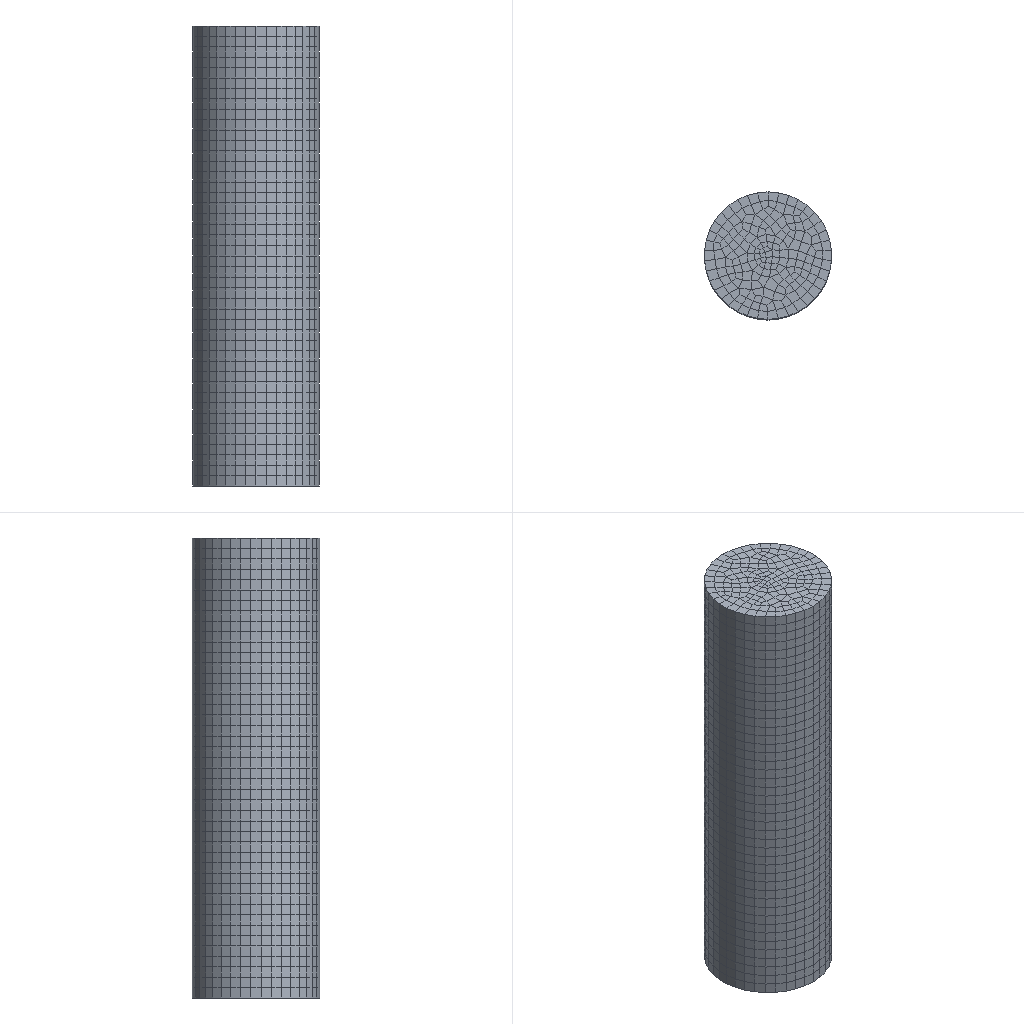Simulation study | abaqus
Set-up summary:
category,name,step,type,value,unit,region
solver,abaqus
solver,version,,,Abaqus/Standard 2020
units,not stated in the deck,,not stated
analysis,deck,,coupled temperature-displacement,coupled temperature-displacement
load_step,Step-1,Step-1,coupled temperature-displacement
load_step,requested,,,1
mesh,nodes,,,9270
mesh,elements,,,8184
element_type,C3D8RT,,solid,8184
load,load commands in deck,,count,2
bc,support commands in deck,,count,1
material,MATERIAL-1,,in results
check,setup vs results,,match,"per instance, exact: element labels, types and connectivity; labels of the nodes the elements use; coordinates of those nodes at SINGLE_PRECISION in 1 of 1 instance(s)"
Abaqus input file, long lists of numbers shortened:
*Heading
** Job name: Job-1 Model name: Model-1
** Generated by: Abaqus/CAE 2020
*Preprint, echo=NO, model=NO, history=NO, contact=NO
**
** PARTS
**
*Part, name=Part-1
*Node
      1,   5.525,  -7.104,          25.
      2,   1.543,  -2.572,          25.
** (9268 more lines like these left out)
*Element, type=C3D8RT
   1, 2958, 2987,  691,  692,  210,  239,   10,   11
   2, 2988, 3021, 3029, 2958,  240,  273,  281,  210
** (8182 more lines like these left out)
*Nset, nset=Set-1, generate
    1,  9270,     1
*Elset, elset=Set-1, generate
    1,  8184,     1
** Section: Section-1
*Solid Section, elset=Set-1, material=Material-1
,
*End Part
**
**
** ASSEMBLY
**
*Assembly, name=Assembly
**
*Instance, name=Part-1-1, part=Part-1
*End Instance
**
*Nset, nset=Set-1, instance=Part-1-1
    2,    5,   46,   47,   48,   49,   50,   51,   52,   53,   54,   55,   56,   57,   58,  109
  110,  111,  112,  113,  114,  115,  116,  117,  118,  119,  120,  121, 1767, 1768, 1769, 1770
** (26 more lines like these left out)
*Elset, elset=Set-1, instance=Part-1-1, generate
 7321,  7640,     1
*Nset, nset=Set-2, instance=Part-1-1
    3,    4,   59,   60,   61,   62,   63,   64,   65,   66,   67,   68,   69,   70,   71,   72
   73,   74,   75,   76,   77,   78,   79,   80,   81,   82,   83,   84,   85,   86,   87,   88
** (11 more lines like these left out)
*Elset, elset=Set-2, instance=Part-1-1
 2465, 2466, 2467, 2468, 2469, 2470, 2471, 2472, 2473, 2474, 2475, 2476, 2477, 2478, 2479, 2480
 2481, 2482, 2483, 2484, 2485, 2486, 2487, 2488, 2489, 2490, 2491, 2492, 2493, 2494, 2495, 2496
** (10 more lines like these left out)
*Elset, elset=_Surf-1_S1, internal, instance=Part-1-1, generate
 7289,  7320,     1
*Surface, type=ELEMENT, name=Surf-1
_Surf-1_S1, S1
*End Assembly
*Amplitude, name=Amp-1, definition=PERIODIC
1,            6.28,              0.,              1.
             1.,              0.
*Amplitude, name=Amp-2
             0.,              0.,             10.,              1.
**
** MATERIALS
**
*Material, name=Material-1
*Conductivity
45.,
*Density
 7.8e-09,
*Elastic
210000., 0.3
*Expansion
 1.5e-05,
*Specific Heat
 4.6e+08,
** ----------------------------------------------------------------
**
** STEP: Step-1
**
*Step, name=Step-1, nlgeom=YES, inc=10000
*Coupled Temperature-displacement, creep=none, deltmx=1e+06, stabilize=0.0002, allsdtol=0.05, continue=NO
1., 1000., 0.01, 1000.
**
** BOUNDARY CONDITIONS
**
** Name: BC-1 Type: 位移/转角
*Boundary
Set-2, 3, 3
**
** LOADS
**
** Name: Load-1   Type: Body heat flux
*Dflux, amplitude=Amp-2
Set-1, BF, 40.
** Name: Load-2   Type: Pressure
*Dsload, amplitude=Amp-1
Surf-1, P, 100.
**
** OUTPUT REQUESTS
**
*Restart, write, frequency=0
**
** FIELD OUTPUT: F-Output-1
**
*Output, field
*Node Output
CF, NT, RF, RFL, RM, RT, TF, U
UR, UT, V, VR, VT
*Element Output, directions=YES
E, HFL, LE, MISES, MISESMAX, MISESONLY, PE, PEEQ, PEEQMAX, PEEQT, PEMAG, S, SF, SSAVG, TEMP, YIELDPOT
*Contact Output
CDISP, CSTRESS
*Radiation Output
FTEMP,
**
** HISTORY OUTPUT: H-Output-1
**
*Output, history, variable=PRESELECT
*End Step
Results summary:
result,step,,completed,increments=17 time=1000.0/1000.0
result,analysis,,,"coupled temperature-displacement, steady state"
result,last_loadstep,,,1
result,primary field,,,"U, NT11"
result,reaction total,,FX,0.0,model units
result,reaction total,,FY,0.0,model units
result,reaction total,,FZ,4.139,model units